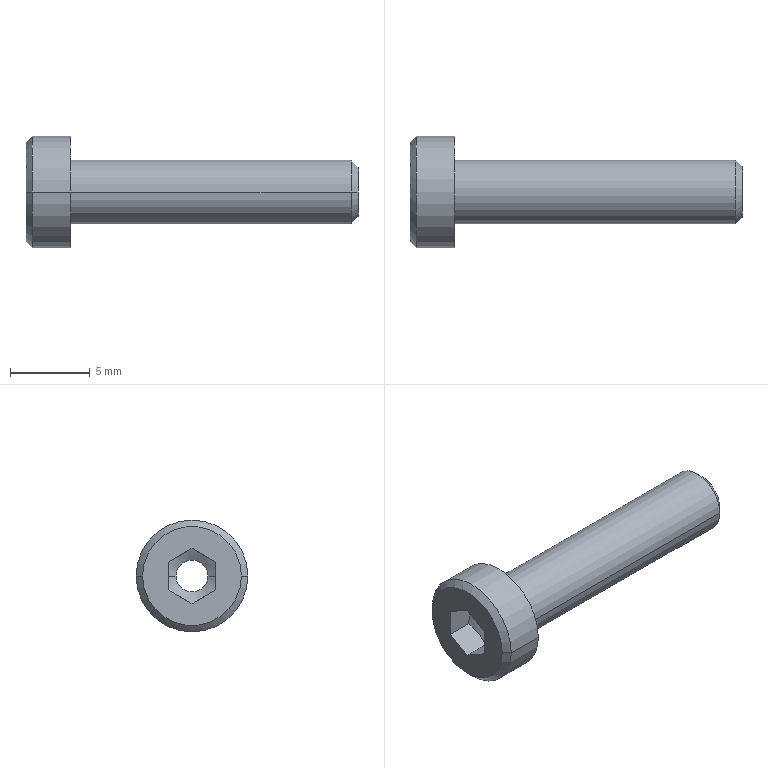Part | STEP file | ASND-0110-Solid1 | 1 solid | 21 faces | box 20.8 x 7 x 7 mm | volume 257.271 mm3 | plane 9 | cylinder 6 | cone 6 | commonest cylinder face diameters 2 x2 4 x2 7 x2